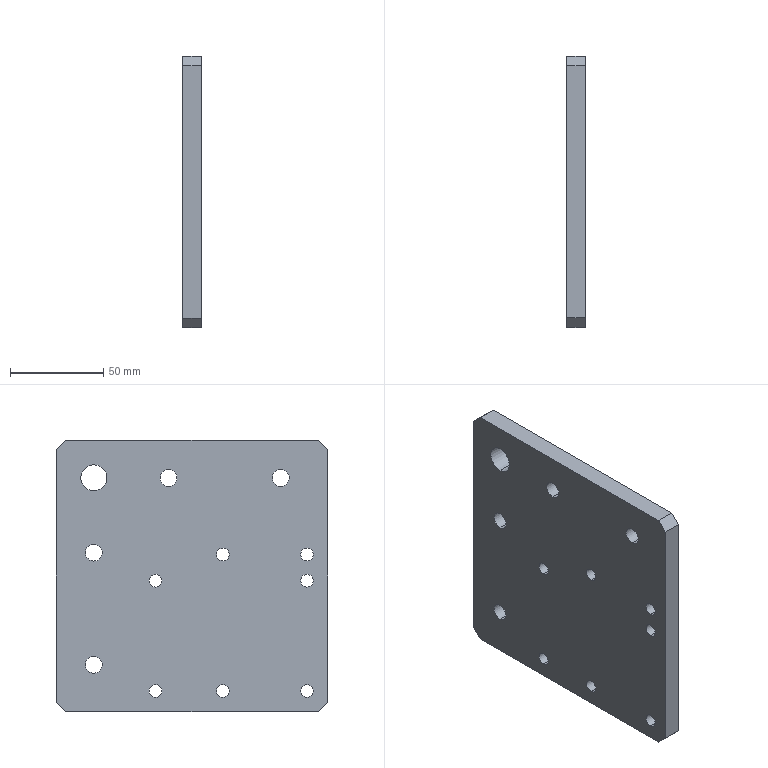Part | SolidWorks | features HoleWzd 2, ICE 2, Chamfer 1, Extrusion 1 | 1 solid | 34 faces | box 10 x 145 x 145 mm | volume 203124 mm3 | cylinder 24 | plane 10 | commonest cylinder face diameters 6.8 x14 9 x8 14 x2
STEP:
#1=CARTESIAN_POINT('',(0.,-47.5,57.));
#2=VERTEX_POINT('',#1);
#3=CARTESIAN_POINT('',(0.,-47.5,48.));
#4=VERTEX_POINT('',#3);
#5=CARTESIAN_POINT('',(0.,-47.5,52.5));
#6=DIRECTION('',(1.,0.,0.));
#7=DIRECTION('',(0.,0.,-1.));
#8=AXIS2_PLACEMENT_3D('',#5,#6,#7);
#9=CIRCLE('',#8,4.5);
#10=EDGE_CURVE('',#2,#4,#9,.T.);
#11=ORIENTED_EDGE('',*,*,#10,.F.);
#12=CARTESIAN_POINT('',(10.,-47.5,57.));
#13=VERTEX_POINT('',#12);
#14=CARTESIAN_POINT('',(0.,-47.5,57.));
#15=DIRECTION('',(1.,0.,0.));
#16=VECTOR('',#15,1000.);
#17=LINE('',#14,#16);
#18=EDGE_CURVE('',#2,#13,#17,.T.);
#19=ORIENTED_EDGE('',*,*,#18,.T.);
#20=CARTESIAN_POINT('',(10.,-47.5,48.));
#21=VERTEX_POINT('',#20);
#22=CARTESIAN_POINT('',(10.,-47.5,52.5));
#23=DIRECTION('',(1.,0.,0.));
#24=DIRECTION('',(0.,0.,-1.));
#25=AXIS2_PLACEMENT_3D('',#22,#23,#24);
#26=CIRCLE('',#25,4.5);
#27=EDGE_CURVE('',#13,#21,#26,.T.);
#28=ORIENTED_EDGE('',*,*,#27,.T.);
#29=CARTESIAN_POINT('',(0.,-47.5,48.));
#30=DIRECTION('',(1.,0.,0.));
#31=VECTOR('',#30,1000.);
#32=LINE('',#29,#31);
#33=EDGE_CURVE('',#4,#21,#32,.T.);
#34=ORIENTED_EDGE('',*,*,#33,.F.);
#35=EDGE_LOOP('',(#11,#19,#28,#34));
#36=FACE_OUTER_BOUND('',#35,.T.);
#37=CARTESIAN_POINT('',(0.,-47.5,52.5));
#38=DIRECTION('',(1.,0.,0.));
#39=DIRECTION('',(0.,0.,-1.));
#40=AXIS2_PLACEMENT_3D('',#37,#38,#39);
#41=CYLINDRICAL_SURFACE('',#40,4.5);
#42=ADVANCED_FACE('',(#36),#41,.F.);
#43=CARTESIAN_POINT('',(0.,12.5,57.));
#44=VERTEX_POINT('',#43);
#45=CARTESIAN_POINT('',(0.,12.5,48.));
#46=VERTEX_POINT('',#45);
#47=CARTESIAN_POINT('',(0.,12.5,52.5));
#48=DIRECTION('',(1.,0.,0.));
#49=DIRECTION('',(0.,0.,-1.));
#50=AXIS2_PLACEMENT_3D('',#47,#48,#49);
#51=CIRCLE('',#50,4.5);
#52=EDGE_CURVE('',#44,#46,#51,.T.);
#53=ORIENTED_EDGE('',*,*,#52,.F.);
#54=CARTESIAN_POINT('',(10.,12.5,57.));
#55=VERTEX_POINT('',#54);
#56=CARTESIAN_POINT('',(0.,12.5,57.));
#57=DIRECTION('',(1.,0.,0.));
#58=VECTOR('',#57,1000.);
#59=LINE('',#56,#58);
#60=EDGE_CURVE('',#44,#55,#59,.T.);
#61=ORIENTED_EDGE('',*,*,#60,.T.);
#62=CARTESIAN_POINT('',(10.,12.5,48.));
#63=VERTEX_POINT('',#62);
#64=CARTESIAN_POINT('',(10.,12.5,52.5));
#65=DIRECTION('',(1.,0.,0.));
#66=DIRECTION('',(0.,0.,-1.));
#67=AXIS2_PLACEMENT_3D('',#64,#65,#66);
#68=CIRCLE('',#67,4.5);
#69=EDGE_CURVE('',#55,#63,#68,.T.);
#70=ORIENTED_EDGE('',*,*,#69,.T.);
#71=CARTESIAN_POINT('',(0.,12.5,48.));
#72=DIRECTION('',(1.,0.,0.));
#73=VECTOR('',#72,1000.);
#74=LINE('',#71,#73);
#75=EDGE_CURVE('',#46,#63,#74,.T.);
#76=ORIENTED_EDGE('',*,*,#75,.F.);
#77=EDGE_LOOP('',(#53,#61,#70,#76));
#78=FACE_OUTER_BOUND('',#77,.T.);
#79=CARTESIAN_POINT('',(0.,12.5,52.5));
#80=DIRECTION('',(1.,0.,0.));
#81=DIRECTION('',(0.,0.,-1.));
#82=AXIS2_PLACEMENT_3D('',#79,#80,#81);
#83=CYLINDRICAL_SURFACE('',#82,4.5);
#84=ADVANCED_FACE('',(#78),#83,.F.);
#85=CARTESIAN_POINT('',(0.,52.5,-43.));
#86=VERTEX_POINT('',#85);
#87=CARTESIAN_POINT('',(0.,52.5,-52.));
#88=VERTEX_POINT('',#87);
#89=CARTESIAN_POINT('',(0.,52.5,-47.5));
#90=DIRECTION('',(1.,0.,0.));
#91=DIRECTION('',(0.,0.,-1.));
#92=AXIS2_PLACEMENT_3D('',#89,#90,#91);
#93=CIRCLE('',#92,4.5);
#94=EDGE_CURVE('',#86,#88,#93,.T.);
#95=ORIENTED_EDGE('',*,*,#94,.F.);
#96=CARTESIAN_POINT('',(10.,52.5,-43.));
#97=VERTEX_POINT('',#96);
#98=CARTESIAN_POINT('',(0.,52.5,-43.));
#99=DIRECTION('',(1.,0.,0.));
#100=VECTOR('',#99,1000.);
#101=LINE('',#98,#100);
#102=EDGE_CURVE('',#86,#97,#101,.T.);
#103=ORIENTED_EDGE('',*,*,#102,.T.);
#104=CARTESIAN_POINT('',(10.,52.5,-52.));
#105=VERTEX_POINT('',#104);
#106=CARTESIAN_POINT('',(10.,52.5,-47.5));
#107=DIRECTION('',(1.,0.,0.));
#108=DIRECTION('',(0.,0.,-1.));
#109=AXIS2_PLACEMENT_3D('',#106,#107,#108);
#110=CIRCLE('',#109,4.5);
#111=EDGE_CURVE('',#97,#105,#110,.T.);
#112=ORIENTED_EDGE('',*,*,#111,.T.);
#113=CARTESIAN_POINT('',(0.,52.5,-52.));
#114=DIRECTION('',(1.,0.,0.));
#115=VECTOR('',#114,1000.);
#116=LINE('',#113,#115);
#117=EDGE_CURVE('',#88,#105,#116,.T.);
#118=ORIENTED_EDGE('',*,*,#117,.F.);
#119=EDGE_LOOP('',(#95,#103,#112,#118));
#120=FACE_OUTER_BOUND('',#119,.T.);
#121=CARTESIAN_POINT('',(0.,52.5,-47.5));
#122=DIRECTION('',(1.,0.,0.));
#123=DIRECTION('',(0.,0.,-1.));
#124=AXIS2_PLACEMENT_3D('',#121,#122,#123);
#125=CYLINDRICAL_SURFACE('',#124,4.5);
#126=ADVANCED_FACE('',(#120),#125,.F.);
#127=CARTESIAN_POINT('',(0.,52.5,17.));
#128=VERTEX_POINT('',#127);
#129=CARTESIAN_POINT('',(0.,52.5,8.));
#130=VERTEX_POINT('',#129);
#131=CARTESIAN_POINT('',(0.,52.5,12.5));
#132=DIRECTION('',(1.,0.,0.));
#133=DIRECTION('',(0.,0.,-1.));
#134=AXIS2_PLACEMENT_3D('',#131,#132,#133);
#135=CIRCLE('',#134,4.5);
#136=EDGE_CURVE('',#128,#130,#135,.T.);
#137=ORIENTED_EDGE('',*,*,#136,.F.);
#138=CARTESIAN_POINT('',(10.,52.5,17.));
#139=VERTEX_POINT('',#138);
#140=CARTESIAN_POINT('',(0.,52.5,17.));
#141=DIRECTION('',(1.,0.,0.));
#142=VECTOR('',#141,1000.);
#143=LINE('',#140,#142);
#144=EDGE_CURVE('',#128,#139,#143,.T.);
#145=ORIENTED_EDGE('',*,*,#144,.T.);
#146=CARTESIAN_POINT('',(10.,52.5,8.));
#147=VERTEX_POINT('',#146);
#148=CARTESIAN_POINT('',(10.,52.5,12.5));
#149=DIRECTION('',(1.,0.,0.));
#150=DIRECTION('',(0.,0.,-1.));
#151=AXIS2_PLACEMENT_3D('',#148,#149,#150);
#152=CIRCLE('',#151,4.5);
#153=EDGE_CURVE('',#139,#147,#152,.T.);
#154=ORIENTED_EDGE('',*,*,#153,.T.);
#155=CARTESIAN_POINT('',(0.,52.5,8.));
#156=DIRECTION('',(1.,0.,0.));
#157=VECTOR('',#156,1000.);
#158=LINE('',#155,#157);
#159=EDGE_CURVE('',#130,#147,#158,.T.);
#160=ORIENTED_EDGE('',*,*,#159,.F.);
#161=EDGE_LOOP('',(#137,#145,#154,#160));
#162=FACE_OUTER_BOUND('',#161,.T.);
#163=CARTESIAN_POINT('',(0.,52.5,12.5));
#164=DIRECTION('',(1.,0.,0.));
#165=DIRECTION('',(0.,0.,-1.));
#166=AXIS2_PLACEMENT_3D('',#163,#164,#165);
#167=CYLINDRICAL_SURFACE('',#166,4.5);
#168=ADVANCED_FACE('',(#162),#167,.F.);
#169=CARTESIAN_POINT('',(0.,52.5,59.5));
#170=VERTEX_POINT('',#169);
#171=CARTESIAN_POINT('',(0.,52.5,45.5));
#172=VERTEX_POINT('',#171);
#173=CARTESIAN_POINT('',(0.,52.5,52.5));
#174=DIRECTION('',(1.,0.,0.));
#175=DIRECTION('',(0.,0.,-1.));
#176=AXIS2_PLACEMENT_3D('',#173,#174,#175);
#177=CIRCLE('',#176,7.);
#178=EDGE_CURVE('',#170,#172,#177,.T.);
#179=ORIENTED_EDGE('',*,*,#178,.F.);
#180=CARTESIAN_POINT('',(10.,52.5,59.5));
#181=VERTEX_POINT('',#180);
#182=CARTESIAN_POINT('',(10.,52.5,59.5));
#183=DIRECTION('',(1.,0.,0.));
#184=VECTOR('',#183,1000.);
#185=LINE('',#182,#184);
#186=EDGE_CURVE('',#170,#181,#185,.T.);
#187=ORIENTED_EDGE('',*,*,#186,.T.);
#188=CARTESIAN_POINT('',(10.,52.5,45.5));
#189=VERTEX_POINT('',#188);
#190=CARTESIAN_POINT('',(10.,52.5,52.5));
#191=DIRECTION('',(1.,0.,0.));
#192=DIRECTION('',(0.,0.,-1.));
#193=AXIS2_PLACEMENT_3D('',#190,#191,#192);
#194=CIRCLE('',#193,7.);
#195=EDGE_CURVE('',#181,#189,#194,.T.);
#196=ORIENTED_EDGE('',*,*,#195,.T.);
#197=CARTESIAN_POINT('',(10.,52.5,45.5));
#198=DIRECTION('',(1.,0.,0.));
#199=VECTOR('',#198,1000.);
#200=LINE('',#197,#199);
#201=EDGE_CURVE('',#172,#189,#200,.T.);
#202=ORIENTED_EDGE('',*,*,#201,.F.);
#203=EDGE_LOOP('',(#179,#187,#196,#202));
#204=FACE_OUTER_BOUND('',#203,.T.);
#205=CARTESIAN_POINT('',(10.,52.5,52.5));
#206=DIRECTION('',(1.,0.,0.));
#207=DIRECTION('',(0.,0.,-1.));
#208=AXIS2_PLACEMENT_3D('',#205,#206,#207);
#209=CYLINDRICAL_SURFACE('',#208,7.);
#210=ADVANCED_FACE('',(#204),#209,.F.);
#211=CARTESIAN_POINT('',(0.,-61.5,-58.1));
#212=VERTEX_POINT('',#211);
#213=CARTESIAN_POINT('',(0.,-61.5,-64.9));
#214=VERTEX_POINT('',#213);
#215=CARTESIAN_POINT('',(0.,-61.5,-61.5));
#216=DIRECTION('',(1.,0.,0.));
#217=DIRECTION('',(0.,0.,-1.));
#218=AXIS2_PLACEMENT_3D('',#215,#216,#217);
#219=CIRCLE('',#218,3.4);
#220=EDGE_CURVE('',#212,#214,#219,.T.);
#221=ORIENTED_EDGE('',*,*,#220,.F.);
#222=CARTESIAN_POINT('',(10.,-61.5,-58.1));
#223=VERTEX_POINT('',#222);
#224=CARTESIAN_POINT('',(10.,-61.5,-58.1));
#225=DIRECTION('',(1.,0.,0.));
#226=VECTOR('',#225,1000.);
#227=LINE('',#224,#226);
#228=EDGE_CURVE('',#212,#223,#227,.T.);
#229=ORIENTED_EDGE('',*,*,#228,.T.);
#230=CARTESIAN_POINT('',(10.,-61.5,-64.9));
#231=VERTEX_POINT('',#230);
#232=CARTESIAN_POINT('',(10.,-61.5,-61.5));
#233=DIRECTION('',(1.,0.,0.));
#234=DIRECTION('',(0.,0.,-1.));
#235=AXIS2_PLACEMENT_3D('',#232,#233,#234);
#236=CIRCLE('',#235,3.4);
#237=EDGE_CURVE('',#223,#231,#236,.T.);
#238=ORIENTED_EDGE('',*,*,#237,.T.);
#239=CARTESIAN_POINT('',(10.,-61.5,-64.9));
#240=DIRECTION('',(1.,0.,0.));
#241=VECTOR('',#240,1000.);
#242=LINE('',#239,#241);
#243=EDGE_CURVE('',#214,#231,#242,.T.);
#244=ORIENTED_EDGE('',*,*,#243,.F.);
#245=EDGE_LOOP('',(#221,#229,#238,#244));
#246=FACE_OUTER_BOUND('',#245,.T.);
#247=CARTESIAN_POINT('',(10.,-61.5,-61.5));
#248=DIRECTION('',(1.,0.,0.));
#249=DIRECTION('',(0.,0.,-1.));
#250=AXIS2_PLACEMENT_3D('',#247,#248,#249);
#251=CYLINDRICAL_SURFACE('',#250,3.4);
#252=ADVANCED_FACE('',(#246),#251,.F.);
#253=CARTESIAN_POINT('',(0.,19.5,0.9));
#254=VERTEX_POINT('',#253);
#255=CARTESIAN_POINT('',(0.,19.5,-5.9));
#256=VERTEX_POINT('',#255);
#257=CARTESIAN_POINT('',(0.,19.5,-2.5));
#258=DIRECTION('',(1.,0.,0.));
#259=DIRECTION('',(0.,0.,-1.));
#260=AXIS2_PLACEMENT_3D('',#257,#258,#259);
#261=CIRCLE('',#260,3.4);
#262=EDGE_CURVE('',#254,#256,#261,.T.);
#263=ORIENTED_EDGE('',*,*,#262,.F.);
#264=CARTESIAN_POINT('',(10.,19.5,0.9));
#265=VERTEX_POINT('',#264);
#266=CARTESIAN_POINT('',(10.,19.5,0.9));
#267=DIRECTION('',(1.,0.,0.));
#268=VECTOR('',#267,1000.);
#269=LINE('',#266,#268);
#270=EDGE_CURVE('',#254,#265,#269,.T.);
#271=ORIENTED_EDGE('',*,*,#270,.T.);
#272=CARTESIAN_POINT('',(10.,19.5,-5.9));
#273=VERTEX_POINT('',#272);
#274=CARTESIAN_POINT('',(10.,19.5,-2.5));
#275=DIRECTION('',(1.,0.,0.));
#276=DIRECTION('',(0.,0.,-1.));
#277=AXIS2_PLACEMENT_3D('',#274,#275,#276);
#278=CIRCLE('',#277,3.4);
#279=EDGE_CURVE('',#265,#273,#278,.T.);
#280=ORIENTED_EDGE('',*,*,#279,.T.);
#281=CARTESIAN_POINT('',(10.,19.5,-5.9));
#282=DIRECTION('',(1.,0.,0.));
#283=VECTOR('',#282,1000.);
#284=LINE('',#281,#283);
#285=EDGE_CURVE('',#256,#273,#284,.T.);
#286=ORIENTED_EDGE('',*,*,#285,.F.);
#287=EDGE_LOOP('',(#263,#271,#280,#286));
#288=FACE_OUTER_BOUND('',#287,.T.);
#289=CARTESIAN_POINT('',(10.,19.5,-2.5));
#290=DIRECTION('',(1.,0.,0.));
#291=DIRECTION('',(0.,0.,-1.));
#292=AXIS2_PLACEMENT_3D('',#289,#290,#291);
#293=CYLINDRICAL_SURFACE('',#292,3.4);
#294=ADVANCED_FACE('',(#288),#293,.F.);
#295=CARTESIAN_POINT('',(0.,19.5,-58.1));
#296=VERTEX_POINT('',#295);
#297=CARTESIAN_POINT('',(0.,19.5,-64.9));
#298=VERTEX_POINT('',#297);
#299=CARTESIAN_POINT('',(0.,19.5,-61.5));
#300=DIRECTION('',(1.,0.,0.));
#301=DIRECTION('',(0.,0.,-1.));
#302=AXIS2_PLACEMENT_3D('',#299,#300,#301);
#303=CIRCLE('',#302,3.4);
#304=EDGE_CURVE('',#296,#298,#303,.T.);
#305=ORIENTED_EDGE('',*,*,#304,.F.);
#306=CARTESIAN_POINT('',(10.,19.5,-58.1));
#307=VERTEX_POINT('',#306);
#308=CARTESIAN_POINT('',(10.,19.5,-58.1));
#309=DIRECTION('',(1.,0.,0.));
#310=VECTOR('',#309,1000.);
#311=LINE('',#308,#310);
#312=EDGE_CURVE('',#296,#307,#311,.T.);
#313=ORIENTED_EDGE('',*,*,#312,.T.);
#314=CARTESIAN_POINT('',(10.,19.5,-64.9));
#315=VERTEX_POINT('',#314);
#316=CARTESIAN_POINT('',(10.,19.5,-61.5));
#317=DIRECTION('',(1.,0.,0.));
#318=DIRECTION('',(0.,0.,-1.));
#319=AXIS2_PLACEMENT_3D('',#316,#317,#318);
#320=CIRCLE('',#319,3.4);
#321=EDGE_CURVE('',#307,#315,#320,.T.);
#322=ORIENTED_EDGE('',*,*,#321,.T.);
#323=CARTESIAN_POINT('',(10.,19.5,-64.9));
#324=DIRECTION('',(1.,0.,0.));
#325=VECTOR('',#324,1000.);
#326=LINE('',#323,#325);
#327=EDGE_CURVE('',#298,#315,#326,.T.);
#328=ORIENTED_EDGE('',*,*,#327,.F.);
#329=EDGE_LOOP('',(#305,#313,#322,#328));
#330=FACE_OUTER_BOUND('',#329,.T.);
#331=CARTESIAN_POINT('',(10.,19.5,-61.5));
#332=DIRECTION('',(1.,0.,0.));
#333=DIRECTION('',(0.,0.,-1.));
#334=AXIS2_PLACEMENT_3D('',#331,#332,#333);
#335=CYLINDRICAL_SURFACE('',#334,3.4);
#336=ADVANCED_FACE('',(#330),#335,.F.);
#337=CARTESIAN_POINT('',(0.,-61.5,0.9));
#338=VERTEX_POINT('',#337);
#339=CARTESIAN_POINT('',(0.,-61.5,-5.9));
#340=VERTEX_POINT('',#339);
#341=CARTESIAN_POINT('',(0.,-61.5,-2.5));
#342=DIRECTION('',(1.,0.,0.));
#343=DIRECTION('',(0.,0.,-1.));
#344=AXIS2_PLACEMENT_3D('',#341,#342,#343);
#345=CIRCLE('',#344,3.4);
#346=EDGE_CURVE('',#338,#340,#345,.T.);
#347=ORIENTED_EDGE('',*,*,#346,.F.);
#348=CARTESIAN_POINT('',(10.,-61.5,0.9));
#349=VERTEX_POINT('',#348);
#350=CARTESIAN_POINT('',(10.,-61.5,0.9));
#351=DIRECTION('',(1.,0.,0.));
#352=VECTOR('',#351,1000.);
#353=LINE('',#350,#352);
#354=EDGE_CURVE('',#338,#349,#353,.T.);
#355=ORIENTED_EDGE('',*,*,#354,.T.);
#356=CARTESIAN_POINT('',(10.,-61.5,-5.9));
#357=VERTEX_POINT('',#356);
#358=CARTESIAN_POINT('',(10.,-61.5,-2.5));
#359=DIRECTION('',(1.,0.,0.));
#360=DIRECTION('',(0.,0.,-1.));
#361=AXIS2_PLACEMENT_3D('',#358,#359,#360);
#362=CIRCLE('',#361,3.4);
#363=EDGE_CURVE('',#349,#357,#362,.T.);
#364=ORIENTED_EDGE('',*,*,#363,.T.);
#365=CARTESIAN_POINT('',(10.,-61.5,-5.9));
#366=DIRECTION('',(1.,0.,0.));
#367=VECTOR('',#366,1000.);
#368=LINE('',#365,#367);
#369=EDGE_CURVE('',#340,#357,#368,.T.);
#370=ORIENTED_EDGE('',*,*,#369,.F.);
#371=EDGE_LOOP('',(#347,#355,#364,#370));
#372=FACE_OUTER_BOUND('',#371,.T.);
#373=CARTESIAN_POINT('',(10.,-61.5,-2.5));
#374=DIRECTION('',(1.,0.,0.));
#375=DIRECTION('',(0.,0.,-1.));
#376=AXIS2_PLACEMENT_3D('',#373,#374,#375);
#377=CYLINDRICAL_SURFACE('',#376,3.4);
#378=ADVANCED_FACE('',(#372),#377,.F.);
#379=CARTESIAN_POINT('',(0.,-61.5,14.9));
#380=VERTEX_POINT('',#379);
#381=CARTESIAN_POINT('',(0.,-61.5,8.1));
#382=VERTEX_POINT('',#381);
#383=CARTESIAN_POINT('',(0.,-61.5,11.5));
#384=DIRECTION('',(1.,0.,0.));
#385=DIRECTION('',(0.,0.,-1.));
#386=AXIS2_PLACEMENT_3D('',#383,#384,#385);
#387=CIRCLE('',#386,3.4);
#388=EDGE_CURVE('',#380,#382,#387,.T.);
#389=ORIENTED_EDGE('',*,*,#388,.F.);
#390=CARTESIAN_POINT('',(10.,-61.5,14.9));
#391=VERTEX_POINT('',#390);
#392=CARTESIAN_POINT('',(10.,-61.5,14.9));
#393=DIRECTION('',(1.,0.,0.));
#394=VECTOR('',#393,1000.);
#395=LINE('',#392,#394);
#396=EDGE_CURVE('',#380,#391,#395,.T.);
#397=ORIENTED_EDGE('',*,*,#396,.T.);
#398=CARTESIAN_POINT('',(10.,-61.5,8.1));
#399=VERTEX_POINT('',#398);
#400=CARTESIAN_POINT('',(10.,-61.5,11.5));
#401=DIRECTION('',(1.,0.,0.));
#402=DIRECTION('',(0.,0.,-1.));
#403=AXIS2_PLACEMENT_3D('',#400,#401,#402);
#404=CIRCLE('',#403,3.4);
#405=EDGE_CURVE('',#391,#399,#404,.T.);
#406=ORIENTED_EDGE('',*,*,#405,.T.);
#407=CARTESIAN_POINT('',(10.,-61.5,8.1));
#408=DIRECTION('',(1.,0.,0.));
#409=VECTOR('',#408,1000.);
#410=LINE('',#407,#409);
#411=EDGE_CURVE('',#382,#399,#410,.T.);
#412=ORIENTED_EDGE('',*,*,#411,.F.);
#413=EDGE_LOOP('',(#389,#397,#406,#412));
#414=FACE_OUTER_BOUND('',#413,.T.);
#415=CARTESIAN_POINT('',(10.,-61.5,11.5));
#416=DIRECTION('',(1.,0.,0.));
#417=DIRECTION('',(0.,0.,-1.));
#418=AXIS2_PLACEMENT_3D('',#415,#416,#417);
#419=CYLINDRICAL_SURFACE('',#418,3.4);
#420=ADVANCED_FACE('',(#414),#419,.F.);
#421=CARTESIAN_POINT('',(0.,-16.5,14.9));
#422=VERTEX_POINT('',#421);
#423=CARTESIAN_POINT('',(0.,-16.5,8.1));
#424=VERTEX_POINT('',#423);
#425=CARTESIAN_POINT('',(0.,-16.5,11.5));
#426=DIRECTION('',(1.,0.,0.));
#427=DIRECTION('',(0.,0.,-1.));
#428=AXIS2_PLACEMENT_3D('',#425,#426,#427);
#429=CIRCLE('',#428,3.4);
#430=EDGE_CURVE('',#422,#424,#429,.T.);
#431=ORIENTED_EDGE('',*,*,#430,.F.);
#432=CARTESIAN_POINT('',(10.,-16.5,14.9));
#433=VERTEX_POINT('',#432);
#434=CARTESIAN_POINT('',(10.,-16.5,14.9));
#435=DIRECTION('',(1.,0.,0.));
#436=VECTOR('',#435,1000.);
#437=LINE('',#434,#436);
#438=EDGE_CURVE('',#422,#433,#437,.T.);
#439=ORIENTED_EDGE('',*,*,#438,.T.);
#440=CARTESIAN_POINT('',(10.,-16.5,8.1));
#441=VERTEX_POINT('',#440);
#442=CARTESIAN_POINT('',(10.,-16.5,11.5));
#443=DIRECTION('',(1.,0.,0.));
#444=DIRECTION('',(0.,0.,-1.));
#445=AXIS2_PLACEMENT_3D('',#442,#443,#444);
#446=CIRCLE('',#445,3.4);
#447=EDGE_CURVE('',#433,#441,#446,.T.);
#448=ORIENTED_EDGE('',*,*,#447,.T.);
#449=CARTESIAN_POINT('',(10.,-16.5,8.1));
#450=DIRECTION('',(1.,0.,0.));
#451=VECTOR('',#450,1000.);
#452=LINE('',#449,#451);
#453=EDGE_CURVE('',#424,#441,#452,.T.);
#454=ORIENTED_EDGE('',*,*,#453,.F.);
#455=EDGE_LOOP('',(#431,#439,#448,#454));
#456=FACE_OUTER_BOUND('',#455,.T.);
#457=CARTESIAN_POINT('',(10.,-16.5,11.5));
#458=DIRECTION('',(1.,0.,0.));
#459=DIRECTION('',(0.,0.,-1.));
#460=AXIS2_PLACEMENT_3D('',#457,#458,#459);
#461=CYLINDRICAL_SURFACE('',#460,3.4);
#462=ADVANCED_FACE('',(#456),#461,.F.);
#463=CARTESIAN_POINT('',(0.,-16.5,-58.1));
#464=VERTEX_POINT('',#463);
#465=CARTESIAN_POINT('',(0.,-16.5,-64.9));
#466=VERTEX_POINT('',#465);
#467=CARTESIAN_POINT('',(0.,-16.5,-61.5));
#468=DIRECTION('',(1.,0.,0.));
#469=DIRECTION('',(0.,0.,-1.));
#470=AXIS2_PLACEMENT_3D('',#467,#468,#469);
#471=CIRCLE('',#470,3.4);
#472=EDGE_CURVE('',#464,#466,#471,.T.);
#473=ORIENTED_EDGE('',*,*,#472,.F.);
#474=CARTESIAN_POINT('',(10.,-16.5,-58.1));
#475=VERTEX_POINT('',#474);
#476=CARTESIAN_POINT('',(10.,-16.5,-58.1));
#477=DIRECTION('',(1.,0.,0.));
#478=VECTOR('',#477,1000.);
#479=LINE('',#476,#478);
#480=EDGE_CURVE('',#464,#475,#479,.T.);
#481=ORIENTED_EDGE('',*,*,#480,.T.);
#482=CARTESIAN_POINT('',(10.,-16.5,-64.9));
#483=VERTEX_POINT('',#482);
#484=CARTESIAN_POINT('',(10.,-16.5,-61.5));
#485=DIRECTION('',(1.,0.,0.));
#486=DIRECTION('',(0.,0.,-1.));
#487=AXIS2_PLACEMENT_3D('',#484,#485,#486);
#488=CIRCLE('',#487,3.4);
#489=EDGE_CURVE('',#475,#483,#488,.T.);
#490=ORIENTED_EDGE('',*,*,#489,.T.);
#491=CARTESIAN_POINT('',(10.,-16.5,-64.9));
#492=DIRECTION('',(1.,0.,0.));
#493=VECTOR('',#492,1000.);
#494=LINE('',#491,#493);
#495=EDGE_CURVE('',#466,#483,#494,.T.);
#496=ORIENTED_EDGE('',*,*,#495,.F.);
#497=EDGE_LOOP('',(#473,#481,#490,#496));
#498=FACE_OUTER_BOUND('',#497,.T.);
#499=CARTESIAN_POINT('',(10.,-16.5,-61.5));
#500=DIRECTION('',(1.,0.,0.));
#501=DIRECTION('',(0.,0.,-1.));
#502=AXIS2_PLACEMENT_3D('',#499,#500,#501);
#503=CYLINDRICAL_SURFACE('',#502,3.4);
#504=ADVANCED_FACE('',(#498),#503,.F.);
#505=CARTESIAN_POINT('',(0.,-67.5,-72.5));
#506=VERTEX_POINT('',#505);
#507=CARTESIAN_POINT('',(0.,67.5,-72.5));
#508=VERTEX_POINT('',#507);
#509=CARTESIAN_POINT('',(0.,-72.5,-72.5));
#510=DIRECTION('',(0.,1.,0.));
#511=VECTOR('',#510,1000.);
#512=LINE('',#509,#511);
#513=EDGE_CURVE('',#506,#508,#512,.T.);
#514=ORIENTED_EDGE('',*,*,#513,.T.);
#515=CARTESIAN_POINT('',(10.,67.5,-72.5));
#516=VERTEX_POINT('',#515);
#517=CARTESIAN_POINT('',(10.,67.5,-72.5));
#518=DIRECTION('',(1.,0.,0.));
#519=VECTOR('',#518,1000.);
#520=LINE('',#517,#519);
#521=EDGE_CURVE('',#508,#516,#520,.T.);
#522=ORIENTED_EDGE('',*,*,#521,.T.);
#523=CARTESIAN_POINT('',(10.,-67.5,-72.5));
#524=VERTEX_POINT('',#523);
#525=CARTESIAN_POINT('',(10.,-72.5,-72.5));
#526=DIRECTION('',(0.,1.,0.));
#527=VECTOR('',#526,1000.);
#528=LINE('',#525,#527);
#529=EDGE_CURVE('',#524,#516,#528,.T.);
#530=ORIENTED_EDGE('',*,*,#529,.F.);
#531=CARTESIAN_POINT('',(10.,-67.5,-72.5));
#532=DIRECTION('',(-1.,0.,0.));
#533=VECTOR('',#532,1000.);
#534=LINE('',#531,#533);
#535=EDGE_CURVE('',#524,#506,#534,.T.);
#536=ORIENTED_EDGE('',*,*,#535,.T.);
#537=EDGE_LOOP('',(#514,#522,#530,#536));
#538=FACE_OUTER_BOUND('',#537,.T.);
#539=CARTESIAN_POINT('',(10.,-72.5,-72.5));
#540=DIRECTION('',(0.,0.,1.));
#541=DIRECTION('',(1.,0.,0.));
#542=AXIS2_PLACEMENT_3D('',#539,#540,#541);
#543=PLANE('',#542);
#544=ADVANCED_FACE('',(#538),#543,.F.);
#545=CARTESIAN_POINT('',(0.,72.5,-67.5));
#546=VERTEX_POINT('',#545);
#547=CARTESIAN_POINT('',(0.,72.5,67.5));
#548=VERTEX_POINT('',#547);
#549=CARTESIAN_POINT('',(0.,72.5,72.5));
#550=DIRECTION('',(0.,0.,1.));
#551=VECTOR('',#550,1000.);
#552=LINE('',#549,#551);
#553=EDGE_CURVE('',#546,#548,#552,.T.);
#554=ORIENTED_EDGE('',*,*,#553,.T.);
#555=CARTESIAN_POINT('',(10.,72.5,67.5));
#556=VERTEX_POINT('',#555);
#557=CARTESIAN_POINT('',(10.,72.5,67.5));
#558=DIRECTION('',(1.,0.,0.));
#559=VECTOR('',#558,1000.);
#560=LINE('',#557,#559);
#561=EDGE_CURVE('',#548,#556,#560,.T.);
#562=ORIENTED_EDGE('',*,*,#561,.T.);
#563=CARTESIAN_POINT('',(10.,72.5,-67.5));
#564=VERTEX_POINT('',#563);
#565=CARTESIAN_POINT('',(10.,72.5,72.5));
#566=DIRECTION('',(0.,0.,1.));
#567=VECTOR('',#566,1000.);
#568=LINE('',#565,#567);
#569=EDGE_CURVE('',#564,#556,#568,.T.);
#570=ORIENTED_EDGE('',*,*,#569,.F.);
#571=CARTESIAN_POINT('',(10.,72.5,-67.5));
#572=DIRECTION('',(-1.,0.,0.));
#573=VECTOR('',#572,1000.);
#574=LINE('',#571,#573);
#575=EDGE_CURVE('',#564,#546,#574,.T.);
#576=ORIENTED_EDGE('',*,*,#575,.T.);
#577=EDGE_LOOP('',(#554,#562,#570,#576));
#578=FACE_OUTER_BOUND('',#577,.T.);
#579=CARTESIAN_POINT('',(10.,72.5,72.5));
#580=DIRECTION('',(0.,-1.,0.));
#581=DIRECTION('',(0.,0.,-1.));
#582=AXIS2_PLACEMENT_3D('',#579,#580,#581);
#583=PLANE('',#582);
#584=ADVANCED_FACE('',(#578),#583,.F.);
#585=CARTESIAN_POINT('',(10.,67.5,72.5));
#586=VERTEX_POINT('',#585);
#587=CARTESIAN_POINT('',(10.,-67.5,72.5));
#588=VERTEX_POINT('',#587);
#589=CARTESIAN_POINT('',(10.,-72.5,72.5));
#590=DIRECTION('',(0.,-1.,0.));
#591=VECTOR('',#590,1000.);
#592=LINE('',#589,#591);
#593=EDGE_CURVE('',#586,#588,#592,.T.);
#594=ORIENTED_EDGE('',*,*,#593,.F.);
#595=CARTESIAN_POINT('',(0.,67.5,72.5));
#596=VERTEX_POINT('',#595);
#597=CARTESIAN_POINT('',(10.,67.5,72.5));
#598=DIRECTION('',(-1.,0.,0.));
#599=VECTOR('',#598,1000.);
#600=LINE('',#597,#599);
#601=EDGE_CURVE('',#586,#596,#600,.T.);
#602=ORIENTED_EDGE('',*,*,#601,.T.);
#603=CARTESIAN_POINT('',(0.,-67.5,72.5));
#604=VERTEX_POINT('',#603);
#605=CARTESIAN_POINT('',(0.,-72.5,72.5));
#606=DIRECTION('',(0.,-1.,0.));
#607=VECTOR('',#606,1000.);
#608=LINE('',#605,#607);
#609=EDGE_CURVE('',#596,#604,#608,.T.);
#610=ORIENTED_EDGE('',*,*,#609,.T.);
#611=CARTESIAN_POINT('',(10.,-67.5,72.5));
#612=DIRECTION('',(1.,0.,0.));
#613=VECTOR('',#612,1000.);
#614=LINE('',#611,#613);
#615=EDGE_CURVE('',#604,#588,#614,.T.);
#616=ORIENTED_EDGE('',*,*,#615,.T.);
#617=EDGE_LOOP('',(#594,#602,#610,#616));
#618=FACE_OUTER_BOUND('',#617,.T.);
#619=CARTESIAN_POINT('',(10.,-72.5,72.5));
#620=DIRECTION('',(0.,0.,-1.));
#621=DIRECTION('',(-1.,0.,0.));
#622=AXIS2_PLACEMENT_3D('',#619,#620,#621);
#623=PLANE('',#622);
#624=ADVANCED_FACE('',(#618),#623,.F.);
#625=CARTESIAN_POINT('',(0.,-72.5,67.5));
#626=VERTEX_POINT('',#625);
#627=CARTESIAN_POINT('',(0.,-72.5,-67.5));
#628=VERTEX_POINT('',#627);
#629=CARTESIAN_POINT('',(0.,-72.5,72.5));
#630=DIRECTION('',(0.,0.,-1.));
#631=VECTOR('',#630,1000.);
#632=LINE('',#629,#631);
#633=EDGE_CURVE('',#626,#628,#632,.T.);
#634=ORIENTED_EDGE('',*,*,#633,.T.);
#635=CARTESIAN_POINT('',(10.,-72.5,-67.5));
#636=VERTEX_POINT('',#635);
#637=CARTESIAN_POINT('',(10.,-72.5,-67.5));
#638=DIRECTION('',(1.,0.,0.));
#639=VECTOR('',#638,1000.);
#640=LINE('',#637,#639);
#641=EDGE_CURVE('',#628,#636,#640,.T.);
#642=ORIENTED_EDGE('',*,*,#641,.T.);
#643=CARTESIAN_POINT('',(10.,-72.5,67.5));
#644=VERTEX_POINT('',#643);
#645=CARTESIAN_POINT('',(10.,-72.5,72.5));
#646=DIRECTION('',(0.,0.,-1.));
#647=VECTOR('',#646,1000.);
#648=LINE('',#645,#647);
#649=EDGE_CURVE('',#644,#636,#648,.T.);
#650=ORIENTED_EDGE('',*,*,#649,.F.);
#651=CARTESIAN_POINT('',(10.,-72.5,67.5));
#652=DIRECTION('',(-1.,0.,0.));
#653=VECTOR('',#652,1000.);
#654=LINE('',#651,#653);
#655=EDGE_CURVE('',#644,#626,#654,.T.);
#656=ORIENTED_EDGE('',*,*,#655,.T.);
#657=EDGE_LOOP('',(#634,#642,#650,#656));
#658=FACE_OUTER_BOUND('',#657,.T.);
#659=CARTESIAN_POINT('',(10.,-72.5,72.5));
#660=DIRECTION('',(0.,1.,0.));
#661=DIRECTION('',(0.,0.,1.));
#662=AXIS2_PLACEMENT_3D('',#659,#660,#661);
#663=PLANE('',#662);
#664=ADVANCED_FACE('',(#658),#663,.F.);
#665=CARTESIAN_POINT('',(10.,-47.5,52.5));
#666=DIRECTION('',(1.,0.,0.));
#667=DIRECTION('',(0.,0.,-1.));
#668=AXIS2_PLACEMENT_3D('',#665,#666,#667);
#669=CIRCLE('',#668,4.5);
#670=EDGE_CURVE('',#21,#13,#669,.T.);
#671=ORIENTED_EDGE('',*,*,#670,.F.);
#672=ORIENTED_EDGE('',*,*,#27,.F.);
#673=EDGE_LOOP('',(#671,#672));
#674=FACE_BOUND('',#673,.T.);
#675=CARTESIAN_POINT('',(10.,12.5,52.5));
#676=DIRECTION('',(1.,0.,0.));
#677=DIRECTION('',(0.,0.,-1.));
#678=AXIS2_PLACEMENT_3D('',#675,#676,#677);
#679=CIRCLE('',#678,4.5);
#680=EDGE_CURVE('',#63,#55,#679,.T.);
#681=ORIENTED_EDGE('',*,*,#680,.F.);
#682=ORIENTED_EDGE('',*,*,#69,.F.);
#683=EDGE_LOOP('',(#681,#682));
#684=FACE_BOUND('',#683,.T.);
#685=CARTESIAN_POINT('',(10.,52.5,-47.5));
#686=DIRECTION('',(1.,0.,0.));
#687=DIRECTION('',(0.,0.,-1.));
#688=AXIS2_PLACEMENT_3D('',#685,#686,#687);
#689=CIRCLE('',#688,4.5);
#690=EDGE_CURVE('',#105,#97,#689,.T.);
#691=ORIENTED_EDGE('',*,*,#690,.F.);
#692=ORIENTED_EDGE('',*,*,#111,.F.);
#693=EDGE_LOOP('',(#691,#692));
#694=FACE_BOUND('',#693,.T.);
#695=CARTESIAN_POINT('',(10.,52.5,12.5));
#696=DIRECTION('',(1.,0.,0.));
#697=DIRECTION('',(0.,0.,-1.));
#698=AXIS2_PLACEMENT_3D('',#695,#696,#697);
#699=CIRCLE('',#698,4.5);
#700=EDGE_CURVE('',#147,#139,#699,.T.);
#701=ORIENTED_EDGE('',*,*,#700,.F.);
#702=ORIENTED_EDGE('',*,*,#153,.F.);
#703=EDGE_LOOP('',(#701,#702));
#704=FACE_BOUND('',#703,.T.);
#705=CARTESIAN_POINT('',(10.,52.5,52.5));
#706=DIRECTION('',(1.,0.,0.));
#707=DIRECTION('',(0.,0.,-1.));
#708=AXIS2_PLACEMENT_3D('',#705,#706,#707);
#709=CIRCLE('',#708,7.);
#710=EDGE_CURVE('',#189,#181,#709,.T.);
#711=ORIENTED_EDGE('',*,*,#710,.F.);
#712=ORIENTED_EDGE('',*,*,#195,.F.);
#713=EDGE_LOOP('',(#711,#712));
#714=FACE_BOUND('',#713,.T.);
#715=CARTESIAN_POINT('',(10.,-61.5,-61.5));
#716=DIRECTION('',(1.,0.,0.));
#717=DIRECTION('',(0.,0.,-1.));
#718=AXIS2_PLACEMENT_3D('',#715,#716,#717);
#719=CIRCLE('',#718,3.4);
#720=EDGE_CURVE('',#231,#223,#719,.T.);
#721=ORIENTED_EDGE('',*,*,#720,.F.);
#722=ORIENTED_EDGE('',*,*,#237,.F.);
#723=EDGE_LOOP('',(#721,#722));
#724=FACE_BOUND('',#723,.T.);
#725=CARTESIAN_POINT('',(10.,19.5,-2.5));
#726=DIRECTION('',(1.,0.,0.));
#727=DIRECTION('',(0.,0.,-1.));
#728=AXIS2_PLACEMENT_3D('',#725,#726,#727);
#729=CIRCLE('',#728,3.4);
#730=EDGE_CURVE('',#273,#265,#729,.T.);
#731=ORIENTED_EDGE('',*,*,#730,.F.);
#732=ORIENTED_EDGE('',*,*,#279,.F.);
#733=EDGE_LOOP('',(#731,#732));
#734=FACE_BOUND('',#733,.T.);
#735=CARTESIAN_POINT('',(10.,19.5,-61.5));
#736=DIRECTION('',(1.,0.,0.));
#737=DIRECTION('',(0.,0.,-1.));
#738=AXIS2_PLACEMENT_3D('',#735,#736,#737);
#739=CIRCLE('',#738,3.4);
#740=EDGE_CURVE('',#315,#307,#739,.T.);
#741=ORIENTED_EDGE('',*,*,#740,.F.);
#742=ORIENTED_EDGE('',*,*,#321,.F.);
#743=EDGE_LOOP('',(#741,#742));
#744=FACE_BOUND('',#743,.T.);
#745=CARTESIAN_POINT('',(10.,-61.5,-2.5));
#746=DIRECTION('',(1.,0.,0.));
#747=DIRECTION('',(0.,0.,-1.));
#748=AXIS2_PLACEMENT_3D('',#745,#746,#747);
#749=CIRCLE('',#748,3.4);
#750=EDGE_CURVE('',#357,#349,#749,.T.);
#751=ORIENTED_EDGE('',*,*,#750,.F.);
#752=ORIENTED_EDGE('',*,*,#363,.F.);
#753=EDGE_LOOP('',(#751,#752));
#754=FACE_BOUND('',#753,.T.);
#755=CARTESIAN_POINT('',(10.,-61.5,11.5));
#756=DIRECTION('',(1.,0.,0.));
#757=DIRECTION('',(0.,0.,-1.));
#758=AXIS2_PLACEMENT_3D('',#755,#756,#757);
#759=CIRCLE('',#758,3.4);
#760=EDGE_CURVE('',#399,#391,#759,.T.);
#761=ORIENTED_EDGE('',*,*,#760,.F.);
#762=ORIENTED_EDGE('',*,*,#405,.F.);
#763=EDGE_LOOP('',(#761,#762));
#764=FACE_BOUND('',#763,.T.);
#765=CARTESIAN_POINT('',(10.,-16.5,11.5));
#766=DIRECTION('',(1.,0.,0.));
#767=DIRECTION('',(0.,0.,-1.));
#768=AXIS2_PLACEMENT_3D('',#765,#766,#767);
#769=CIRCLE('',#768,3.4);
#770=EDGE_CURVE('',#441,#433,#769,.T.);
#771=ORIENTED_EDGE('',*,*,#770,.F.);
#772=ORIENTED_EDGE('',*,*,#447,.F.);
#773=EDGE_LOOP('',(#771,#772));
#774=FACE_BOUND('',#773,.T.);
#775=CARTESIAN_POINT('',(10.,-16.5,-61.5));
#776=DIRECTION('',(1.,0.,0.));
#777=DIRECTION('',(0.,0.,-1.));
#778=AXIS2_PLACEMENT_3D('',#775,#776,#777);
#779=CIRCLE('',#778,3.4);
#780=EDGE_CURVE('',#483,#475,#779,.T.);
#781=ORIENTED_EDGE('',*,*,#780,.F.);
#782=ORIENTED_EDGE('',*,*,#489,.F.);
#783=EDGE_LOOP('',(#781,#782));
#784=FACE_BOUND('',#783,.T.);
#785=ORIENTED_EDGE('',*,*,#569,.T.);
#786=CARTESIAN_POINT('',(10.,67.5,72.5));
#787=DIRECTION('',(0.,-0.7071,0.7071));
#788=VECTOR('',#787,1000.);
#789=LINE('',#786,#788);
#790=EDGE_CURVE('',#556,#586,#789,.T.);
#791=ORIENTED_EDGE('',*,*,#790,.T.);
#792=ORIENTED_EDGE('',*,*,#593,.T.);
#793=CARTESIAN_POINT('',(10.,-72.5,67.5));
#794=DIRECTION('',(0.,-0.7071,-0.7071));
#795=VECTOR('',#794,1000.);
#796=LINE('',#793,#795);
#797=EDGE_CURVE('',#588,#644,#796,.T.);
#798=ORIENTED_EDGE('',*,*,#797,.T.);
#799=ORIENTED_EDGE('',*,*,#649,.T.);
#800=CARTESIAN_POINT('',(10.,-67.5,-72.5));
#801=DIRECTION('',(0.,0.7071,-0.7071));
#802=VECTOR('',#801,1000.);
#803=LINE('',#800,#802);
#804=EDGE_CURVE('',#636,#524,#803,.T.);
#805=ORIENTED_EDGE('',*,*,#804,.T.);
#806=ORIENTED_EDGE('',*,*,#529,.T.);
#807=CARTESIAN_POINT('',(10.,72.5,-67.5));
#808=DIRECTION('',(0.,0.7071,0.7071));
#809=VECTOR('',#808,1000.);
#810=LINE('',#807,#809);
#811=EDGE_CURVE('',#516,#564,#810,.T.);
#812=ORIENTED_EDGE('',*,*,#811,.T.);
#813=EDGE_LOOP('',(#785,#791,#792,#798,#799,#805,#806,#812));
#814=FACE_OUTER_BOUND('',#813,.T.);
#815=CARTESIAN_POINT('',(10.,0.,0.));
#816=DIRECTION('',(-1.,0.,0.));
#817=DIRECTION('',(0.,0.,1.));
#818=AXIS2_PLACEMENT_3D('',#815,#816,#817);
#819=PLANE('',#818);
#820=ADVANCED_FACE('',(#674,#684,#694,#704,#714,#724,#734,#744,#754,#764,#774,#784,#814),#819,.F.);
#821=CARTESIAN_POINT('',(0.,-47.5,52.5));
#822=DIRECTION('',(1.,0.,0.));
#823=DIRECTION('',(0.,0.,-1.));
#824=AXIS2_PLACEMENT_3D('',#821,#822,#823);
#825=CIRCLE('',#824,4.5);
#826=EDGE_CURVE('',#4,#2,#825,.T.);
#827=ORIENTED_EDGE('',*,*,#826,.T.);
#828=ORIENTED_EDGE('',*,*,#10,.T.);
#829=EDGE_LOOP('',(#827,#828));
#830=FACE_BOUND('',#829,.T.);
#831=CARTESIAN_POINT('',(0.,12.5,52.5));
#832=DIRECTION('',(1.,0.,0.));
#833=DIRECTION('',(0.,0.,-1.));
#834=AXIS2_PLACEMENT_3D('',#831,#832,#833);
#835=CIRCLE('',#834,4.5);
#836=EDGE_CURVE('',#46,#44,#835,.T.);
#837=ORIENTED_EDGE('',*,*,#836,.T.);
#838=ORIENTED_EDGE('',*,*,#52,.T.);
#839=EDGE_LOOP('',(#837,#838));
#840=FACE_BOUND('',#839,.T.);
#841=CARTESIAN_POINT('',(0.,52.5,-47.5));
#842=DIRECTION('',(1.,0.,0.));
#843=DIRECTION('',(0.,0.,-1.));
#844=AXIS2_PLACEMENT_3D('',#841,#842,#843);
#845=CIRCLE('',#844,4.5);
#846=EDGE_CURVE('',#88,#86,#845,.T.);
#847=ORIENTED_EDGE('',*,*,#846,.T.);
#848=ORIENTED_EDGE('',*,*,#94,.T.);
#849=EDGE_LOOP('',(#847,#848));
#850=FACE_BOUND('',#849,.T.);
#851=CARTESIAN_POINT('',(0.,52.5,12.5));
#852=DIRECTION('',(1.,0.,0.));
#853=DIRECTION('',(0.,0.,-1.));
#854=AXIS2_PLACEMENT_3D('',#851,#852,#853);
#855=CIRCLE('',#854,4.5);
#856=EDGE_CURVE('',#130,#128,#855,.T.);
#857=ORIENTED_EDGE('',*,*,#856,.T.);
#858=ORIENTED_EDGE('',*,*,#136,.T.);
#859=EDGE_LOOP('',(#857,#858));
#860=FACE_BOUND('',#859,.T.);
#861=CARTESIAN_POINT('',(0.,52.5,52.5));
#862=DIRECTION('',(1.,0.,0.));
#863=DIRECTION('',(0.,0.,-1.));
#864=AXIS2_PLACEMENT_3D('',#861,#862,#863);
#865=CIRCLE('',#864,7.);
#866=EDGE_CURVE('',#172,#170,#865,.T.);
#867=ORIENTED_EDGE('',*,*,#866,.T.);
#868=ORIENTED_EDGE('',*,*,#178,.T.);
#869=EDGE_LOOP('',(#867,#868));
#870=FACE_BOUND('',#869,.T.);
#871=CARTESIAN_POINT('',(0.,-61.5,-61.5));
#872=DIRECTION('',(1.,0.,0.));
#873=DIRECTION('',(0.,0.,-1.));
#874=AXIS2_PLACEMENT_3D('',#871,#872,#873);
#875=CIRCLE('',#874,3.4);
#876=EDGE_CURVE('',#214,#212,#875,.T.);
#877=ORIENTED_EDGE('',*,*,#876,.T.);
#878=ORIENTED_EDGE('',*,*,#220,.T.);
#879=EDGE_LOOP('',(#877,#878));
#880=FACE_BOUND('',#879,.T.);
#881=CARTESIAN_POINT('',(0.,19.5,-2.5));
#882=DIRECTION('',(1.,0.,0.));
#883=DIRECTION('',(0.,0.,-1.));
#884=AXIS2_PLACEMENT_3D('',#881,#882,#883);
#885=CIRCLE('',#884,3.4);
#886=EDGE_CURVE('',#256,#254,#885,.T.);
#887=ORIENTED_EDGE('',*,*,#886,.T.);
#888=ORIENTED_EDGE('',*,*,#262,.T.);
#889=EDGE_LOOP('',(#887,#888));
#890=FACE_BOUND('',#889,.T.);
#891=CARTESIAN_POINT('',(0.,19.5,-61.5));
#892=DIRECTION('',(1.,0.,0.));
#893=DIRECTION('',(0.,0.,-1.));
#894=AXIS2_PLACEMENT_3D('',#891,#892,#893);
#895=CIRCLE('',#894,3.4);
#896=EDGE_CURVE('',#298,#296,#895,.T.);
#897=ORIENTED_EDGE('',*,*,#896,.T.);
#898=ORIENTED_EDGE('',*,*,#304,.T.);
#899=EDGE_LOOP('',(#897,#898));
#900=FACE_BOUND('',#899,.T.);
#901=CARTESIAN_POINT('',(0.,-61.5,-2.5));
#902=DIRECTION('',(1.,0.,0.));
#903=DIRECTION('',(0.,0.,-1.));
#904=AXIS2_PLACEMENT_3D('',#901,#902,#903);
#905=CIRCLE('',#904,3.4);
#906=EDGE_CURVE('',#340,#338,#905,.T.);
#907=ORIENTED_EDGE('',*,*,#906,.T.);
#908=ORIENTED_EDGE('',*,*,#346,.T.);
#909=EDGE_LOOP('',(#907,#908));
#910=FACE_BOUND('',#909,.T.);
#911=CARTESIAN_POINT('',(0.,-61.5,11.5));
#912=DIRECTION('',(1.,0.,0.));
#913=DIRECTION('',(0.,0.,-1.));
#914=AXIS2_PLACEMENT_3D('',#911,#912,#913);
#915=CIRCLE('',#914,3.4);
#916=EDGE_CURVE('',#382,#380,#915,.T.);
#917=ORIENTED_EDGE('',*,*,#916,.T.);
#918=ORIENTED_EDGE('',*,*,#388,.T.);
#919=EDGE_LOOP('',(#917,#918));
#920=FACE_BOUND('',#919,.T.);
#921=CARTESIAN_POINT('',(0.,-16.5,11.5));
#922=DIRECTION('',(1.,0.,0.));
#923=DIRECTION('',(0.,0.,-1.));
#924=AXIS2_PLACEMENT_3D('',#921,#922,#923);
#925=CIRCLE('',#924,3.4);
#926=EDGE_CURVE('',#424,#422,#925,.T.);
#927=ORIENTED_EDGE('',*,*,#926,.T.);
#928=ORIENTED_EDGE('',*,*,#430,.T.);
#929=EDGE_LOOP('',(#927,#928));
#930=FACE_BOUND('',#929,.T.);
#931=CARTESIAN_POINT('',(0.,-16.5,-61.5));
#932=DIRECTION('',(1.,0.,0.));
#933=DIRECTION('',(0.,0.,-1.));
#934=AXIS2_PLACEMENT_3D('',#931,#932,#933);
#935=CIRCLE('',#934,3.4);
#936=EDGE_CURVE('',#466,#464,#935,.T.);
#937=ORIENTED_EDGE('',*,*,#936,.T.);
#938=ORIENTED_EDGE('',*,*,#472,.T.);
#939=EDGE_LOOP('',(#937,#938));
#940=FACE_BOUND('',#939,.T.);
#941=ORIENTED_EDGE('',*,*,#609,.F.);
#942=CARTESIAN_POINT('',(0.,70.,70.));
#943=DIRECTION('',(0.,0.7071,-0.7071));
#944=VECTOR('',#943,1000.);
#945=LINE('',#942,#944);
#946=EDGE_CURVE('',#596,#548,#945,.T.);
#947=ORIENTED_EDGE('',*,*,#946,.T.);
#948=ORIENTED_EDGE('',*,*,#553,.F.);
#949=CARTESIAN_POINT('',(0.,70.,-70.));
#950=DIRECTION('',(0.,-0.7071,-0.7071));
#951=VECTOR('',#950,1000.);
#952=LINE('',#949,#951);
#953=EDGE_CURVE('',#546,#508,#952,.T.);
#954=ORIENTED_EDGE('',*,*,#953,.T.);
#955=ORIENTED_EDGE('',*,*,#513,.F.);
#956=CARTESIAN_POINT('',(0.,-70.,-70.));
#957=DIRECTION('',(0.,-0.7071,0.7071));
#958=VECTOR('',#957,1000.);
#959=LINE('',#956,#958);
#960=EDGE_CURVE('',#506,#628,#959,.T.);
#961=ORIENTED_EDGE('',*,*,#960,.T.);
#962=ORIENTED_EDGE('',*,*,#633,.F.);
#963=CARTESIAN_POINT('',(0.,-70.,70.));
#964=DIRECTION('',(0.,0.7071,0.7071));
#965=VECTOR('',#964,1000.);
#966=LINE('',#963,#965);
#967=EDGE_CURVE('',#626,#604,#966,.T.);
#968=ORIENTED_EDGE('',*,*,#967,.T.);
#969=EDGE_LOOP('',(#941,#947,#948,#954,#955,#961,#962,#968));
#970=FACE_OUTER_BOUND('',#969,.T.);
#971=CARTESIAN_POINT('',(0.,0.,0.));
#972=DIRECTION('',(-1.,0.,0.));
#973=DIRECTION('',(0.,0.,1.));
#974=AXIS2_PLACEMENT_3D('',#971,#972,#973);
#975=PLANE('',#974);
#976=ADVANCED_FACE('',(#830,#840,#850,#860,#870,#880,#890,#900,#910,#920,#930,#940,#970),#975,.T.);
#977=ORIENTED_EDGE('',*,*,#790,.F.);
#978=ORIENTED_EDGE('',*,*,#561,.F.);
#979=ORIENTED_EDGE('',*,*,#946,.F.);
#980=ORIENTED_EDGE('',*,*,#601,.F.);
#981=EDGE_LOOP('',(#977,#978,#979,#980));
#982=FACE_OUTER_BOUND('',#981,.T.);
#983=CARTESIAN_POINT('',(10.,67.5,72.5));
#984=DIRECTION('',(0.,-0.7071,-0.7071));
#985=DIRECTION('',(-1.,0.,0.));
#986=AXIS2_PLACEMENT_3D('',#983,#984,#985);
#987=PLANE('',#986);
#988=ADVANCED_FACE('',(#982),#987,.F.);
#989=ORIENTED_EDGE('',*,*,#811,.F.);
#990=ORIENTED_EDGE('',*,*,#521,.F.);
#991=ORIENTED_EDGE('',*,*,#953,.F.);
#992=ORIENTED_EDGE('',*,*,#575,.F.);
#993=EDGE_LOOP('',(#989,#990,#991,#992));
#994=FACE_OUTER_BOUND('',#993,.T.);
#995=CARTESIAN_POINT('',(10.,72.5,-67.5));
#996=DIRECTION('',(0.,-0.7071,0.7071));
#997=DIRECTION('',(-1.,0.,0.));
#998=AXIS2_PLACEMENT_3D('',#995,#996,#997);
#999=PLANE('',#998);
#1000=ADVANCED_FACE('',(#994),#999,.F.);
#1001=ORIENTED_EDGE('',*,*,#804,.F.);
#1002=ORIENTED_EDGE('',*,*,#641,.F.);
#1003=ORIENTED_EDGE('',*,*,#960,.F.);
#1004=ORIENTED_EDGE('',*,*,#535,.F.);
#1005=EDGE_LOOP('',(#1001,#1002,#1003,#1004));
#1006=FACE_OUTER_BOUND('',#1005,.T.);
#1007=CARTESIAN_POINT('',(10.,-67.5,-72.5));
#1008=DIRECTION('',(0.,0.7071,0.7071));
#1009=DIRECTION('',(-1.,0.,0.));
#1010=AXIS2_PLACEMENT_3D('',#1007,#1008,#1009);
#1011=PLANE('',#1010);
#1012=ADVANCED_FACE('',(#1006),#1011,.F.);
#1013=ORIENTED_EDGE('',*,*,#797,.F.);
#1014=ORIENTED_EDGE('',*,*,#615,.F.);
#1015=ORIENTED_EDGE('',*,*,#967,.F.);
#1016=ORIENTED_EDGE('',*,*,#655,.F.);
#1017=EDGE_LOOP('',(#1013,#1014,#1015,#1016));
#1018=FACE_OUTER_BOUND('',#1017,.T.);
#1019=CARTESIAN_POINT('',(10.,-72.5,67.5));
#1020=DIRECTION('',(0.,0.7071,-0.7071));
#1021=DIRECTION('',(-1.,0.,0.));
#1022=AXIS2_PLACEMENT_3D('',#1019,#1020,#1021);
#1023=PLANE('',#1022);
#1024=ADVANCED_FACE('',(#1018),#1023,.F.);
#1025=ORIENTED_EDGE('',*,*,#480,.F.);
#1026=ORIENTED_EDGE('',*,*,#936,.F.);
#1027=ORIENTED_EDGE('',*,*,#495,.T.);
#1028=ORIENTED_EDGE('',*,*,#780,.T.);
#1029=EDGE_LOOP('',(#1025,#1026,#1027,#1028));
#1030=FACE_OUTER_BOUND('',#1029,.T.);
#1031=CARTESIAN_POINT('',(10.,-16.5,-61.5));
#1032=DIRECTION('',(1.,0.,0.));
#1033=DIRECTION('',(0.,0.,-1.));
#1034=AXIS2_PLACEMENT_3D('',#1031,#1032,#1033);
#1035=CYLINDRICAL_SURFACE('',#1034,3.4);
#1036=ADVANCED_FACE('',(#1030),#1035,.F.);
#1037=ORIENTED_EDGE('',*,*,#438,.F.);
#1038=ORIENTED_EDGE('',*,*,#926,.F.);
#1039=ORIENTED_EDGE('',*,*,#453,.T.);
#1040=ORIENTED_EDGE('',*,*,#770,.T.);
#1041=EDGE_LOOP('',(#1037,#1038,#1039,#1040));
#1042=FACE_OUTER_BOUND('',#1041,.T.);
#1043=CARTESIAN_POINT('',(10.,-16.5,11.5));
#1044=DIRECTION('',(1.,0.,0.));
#1045=DIRECTION('',(0.,0.,-1.));
#1046=AXIS2_PLACEMENT_3D('',#1043,#1044,#1045);
#1047=CYLINDRICAL_SURFACE('',#1046,3.4);
#1048=ADVANCED_FACE('',(#1042),#1047,.F.);
#1049=ORIENTED_EDGE('',*,*,#396,.F.);
#1050=ORIENTED_EDGE('',*,*,#916,.F.);
#1051=ORIENTED_EDGE('',*,*,#411,.T.);
#1052=ORIENTED_EDGE('',*,*,#760,.T.);
#1053=EDGE_LOOP('',(#1049,#1050,#1051,#1052));
#1054=FACE_OUTER_BOUND('',#1053,.T.);
#1055=CARTESIAN_POINT('',(10.,-61.5,11.5));
#1056=DIRECTION('',(1.,0.,0.));
#1057=DIRECTION('',(0.,0.,-1.));
#1058=AXIS2_PLACEMENT_3D('',#1055,#1056,#1057);
#1059=CYLINDRICAL_SURFACE('',#1058,3.4);
#1060=ADVANCED_FACE('',(#1054),#1059,.F.);
#1061=ORIENTED_EDGE('',*,*,#354,.F.);
#1062=ORIENTED_EDGE('',*,*,#906,.F.);
#1063=ORIENTED_EDGE('',*,*,#369,.T.);
#1064=ORIENTED_EDGE('',*,*,#750,.T.);
#1065=EDGE_LOOP('',(#1061,#1062,#1063,#1064));
#1066=FACE_OUTER_BOUND('',#1065,.T.);
#1067=CARTESIAN_POINT('',(10.,-61.5,-2.5));
#1068=DIRECTION('',(1.,0.,0.));
#1069=DIRECTION('',(0.,0.,-1.));
#1070=AXIS2_PLACEMENT_3D('',#1067,#1068,#1069);
#1071=CYLINDRICAL_SURFACE('',#1070,3.4);
#1072=ADVANCED_FACE('',(#1066),#1071,.F.);
#1073=ORIENTED_EDGE('',*,*,#312,.F.);
#1074=ORIENTED_EDGE('',*,*,#896,.F.);
#1075=ORIENTED_EDGE('',*,*,#327,.T.);
#1076=ORIENTED_EDGE('',*,*,#740,.T.);
#1077=EDGE_LOOP('',(#1073,#1074,#1075,#1076));
#1078=FACE_OUTER_BOUND('',#1077,.T.);
#1079=CARTESIAN_POINT('',(10.,19.5,-61.5));
#1080=DIRECTION('',(1.,0.,0.));
#1081=DIRECTION('',(0.,0.,-1.));
#1082=AXIS2_PLACEMENT_3D('',#1079,#1080,#1081);
#1083=CYLINDRICAL_SURFACE('',#1082,3.4);
#1084=ADVANCED_FACE('',(#1078),#1083,.F.);
#1085=ORIENTED_EDGE('',*,*,#270,.F.);
#1086=ORIENTED_EDGE('',*,*,#886,.F.);
#1087=ORIENTED_EDGE('',*,*,#285,.T.);
#1088=ORIENTED_EDGE('',*,*,#730,.T.);
#1089=EDGE_LOOP('',(#1085,#1086,#1087,#1088));
#1090=FACE_OUTER_BOUND('',#1089,.T.);
#1091=CARTESIAN_POINT('',(10.,19.5,-2.5));
#1092=DIRECTION('',(1.,0.,0.));
#1093=DIRECTION('',(0.,0.,-1.));
#1094=AXIS2_PLACEMENT_3D('',#1091,#1092,#1093);
#1095=CYLINDRICAL_SURFACE('',#1094,3.4);
#1096=ADVANCED_FACE('',(#1090),#1095,.F.);
#1097=ORIENTED_EDGE('',*,*,#228,.F.);
#1098=ORIENTED_EDGE('',*,*,#876,.F.);
#1099=ORIENTED_EDGE('',*,*,#243,.T.);
#1100=ORIENTED_EDGE('',*,*,#720,.T.);
#1101=EDGE_LOOP('',(#1097,#1098,#1099,#1100));
#1102=FACE_OUTER_BOUND('',#1101,.T.);
#1103=CARTESIAN_POINT('',(10.,-61.5,-61.5));
#1104=DIRECTION('',(1.,0.,0.));
#1105=DIRECTION('',(0.,0.,-1.));
#1106=AXIS2_PLACEMENT_3D('',#1103,#1104,#1105);
#1107=CYLINDRICAL_SURFACE('',#1106,3.4);
#1108=ADVANCED_FACE('',(#1102),#1107,.F.);
#1109=ORIENTED_EDGE('',*,*,#186,.F.);
#1110=ORIENTED_EDGE('',*,*,#866,.F.);
#1111=ORIENTED_EDGE('',*,*,#201,.T.);
#1112=ORIENTED_EDGE('',*,*,#710,.T.);
#1113=EDGE_LOOP('',(#1109,#1110,#1111,#1112));
#1114=FACE_OUTER_BOUND('',#1113,.T.);
#1115=CARTESIAN_POINT('',(10.,52.5,52.5));
#1116=DIRECTION('',(1.,0.,0.));
#1117=DIRECTION('',(0.,0.,-1.));
#1118=AXIS2_PLACEMENT_3D('',#1115,#1116,#1117);
#1119=CYLINDRICAL_SURFACE('',#1118,7.);
#1120=ADVANCED_FACE('',(#1114),#1119,.F.);
#1121=ORIENTED_EDGE('',*,*,#144,.F.);
#1122=ORIENTED_EDGE('',*,*,#856,.F.);
#1123=ORIENTED_EDGE('',*,*,#159,.T.);
#1124=ORIENTED_EDGE('',*,*,#700,.T.);
#1125=EDGE_LOOP('',(#1121,#1122,#1123,#1124));
#1126=FACE_OUTER_BOUND('',#1125,.T.);
#1127=CARTESIAN_POINT('',(0.,52.5,12.5));
#1128=DIRECTION('',(1.,0.,0.));
#1129=DIRECTION('',(0.,0.,-1.));
#1130=AXIS2_PLACEMENT_3D('',#1127,#1128,#1129);
#1131=CYLINDRICAL_SURFACE('',#1130,4.5);
#1132=ADVANCED_FACE('',(#1126),#1131,.F.);
#1133=ORIENTED_EDGE('',*,*,#102,.F.);
#1134=ORIENTED_EDGE('',*,*,#846,.F.);
#1135=ORIENTED_EDGE('',*,*,#117,.T.);
#1136=ORIENTED_EDGE('',*,*,#690,.T.);
#1137=EDGE_LOOP('',(#1133,#1134,#1135,#1136));
#1138=FACE_OUTER_BOUND('',#1137,.T.);
#1139=CARTESIAN_POINT('',(0.,52.5,-47.5));
#1140=DIRECTION('',(1.,0.,0.));
#1141=DIRECTION('',(0.,0.,-1.));
#1142=AXIS2_PLACEMENT_3D('',#1139,#1140,#1141);
#1143=CYLINDRICAL_SURFACE('',#1142,4.5);
#1144=ADVANCED_FACE('',(#1138),#1143,.F.);
#1145=ORIENTED_EDGE('',*,*,#60,.F.);
#1146=ORIENTED_EDGE('',*,*,#836,.F.);
#1147=ORIENTED_EDGE('',*,*,#75,.T.);
#1148=ORIENTED_EDGE('',*,*,#680,.T.);
#1149=EDGE_LOOP('',(#1145,#1146,#1147,#1148));
#1150=FACE_OUTER_BOUND('',#1149,.T.);
#1151=CARTESIAN_POINT('',(0.,12.5,52.5));
#1152=DIRECTION('',(1.,0.,0.));
#1153=DIRECTION('',(0.,0.,-1.));
#1154=AXIS2_PLACEMENT_3D('',#1151,#1152,#1153);
#1155=CYLINDRICAL_SURFACE('',#1154,4.5);
#1156=ADVANCED_FACE('',(#1150),#1155,.F.);
#1157=ORIENTED_EDGE('',*,*,#18,.F.);
#1158=ORIENTED_EDGE('',*,*,#826,.F.);
#1159=ORIENTED_EDGE('',*,*,#33,.T.);
#1160=ORIENTED_EDGE('',*,*,#670,.T.);
#1161=EDGE_LOOP('',(#1157,#1158,#1159,#1160));
#1162=FACE_OUTER_BOUND('',#1161,.T.);
#1163=CARTESIAN_POINT('',(0.,-47.5,52.5));
#1164=DIRECTION('',(1.,0.,0.));
#1165=DIRECTION('',(0.,0.,-1.));
#1166=AXIS2_PLACEMENT_3D('',#1163,#1164,#1165);
#1167=CYLINDRICAL_SURFACE('',#1166,4.5);
#1168=ADVANCED_FACE('',(#1162),#1167,.F.);
#1169=CLOSED_SHELL('',(#42,#84,#126,#168,#210,#252,#294,#336,#378,#420,#462,#504,#544,#584,#624,#664,#820,#976,#988,#1000,#1012,#1024,#1036,#1048,#1060,#1072,#1084,#1096,#1108,#1120,#1132,#1144,#1156,#1168));
#1170=MANIFOLD_SOLID_BREP('',#1169);
#1171=CARTESIAN_POINT('',(0.,0.,0.));
#1172=DIRECTION('',(0.,0.,1.));
#1173=DIRECTION('',(1.,0.,0.));
#1174=AXIS2_PLACEMENT_3D('',#1171,#1172,#1173);
#1175=(LENGTH_UNIT()NAMED_UNIT(*)SI_UNIT(.MILLI.,.METRE.));
#1176=UNCERTAINTY_MEASURE_WITH_UNIT(LENGTH_MEASURE(0.00001),#1175,'','');
#1177=(NAMED_UNIT(*)PLANE_ANGLE_UNIT()SI_UNIT($,.RADIAN.));
#1178=(NAMED_UNIT(*)SI_UNIT($,.STERADIAN.)SOLID_ANGLE_UNIT());
#1179=(GEOMETRIC_REPRESENTATION_CONTEXT(3)GLOBAL_UNCERTAINTY_ASSIGNED_CONTEXT((#1176))GLOBAL_UNIT_ASSIGNED_CONTEXT((#1175,#1177,#1178))REPRESENTATION_CONTEXT('',''));
#1180=ADVANCED_BREP_SHAPE_REPRESENTATION('',(#1170,#1174),#1179);